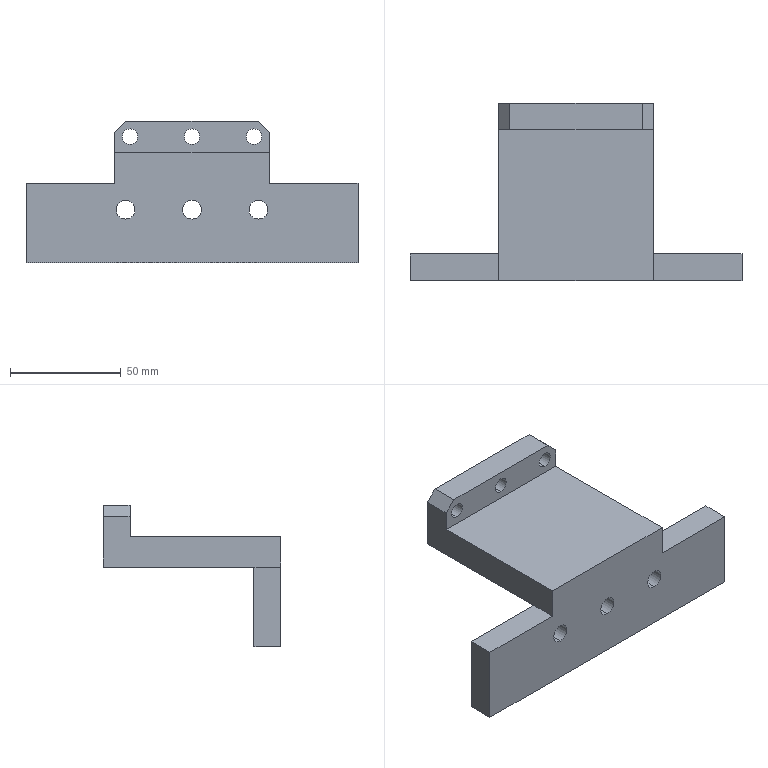NC program | NX | posted with a generic post | part box 150 x 80 x 64 mm
Lines 1 to 22 of 10576:
N10 G17 G21 G94 G90
(FLOOR_WALL , TOOL : D63)
N12 T01 M6
N14 G54
N16 G17 G0 G90 X-113. Y43.497 B0. C0. S6500 M3
N18 G43 Z30. H1
N20 Z3.
N22 G94 G1 Z0. F1250.
N24 X-110.
N26 X110.
N28 Y12.599
N30 X-110.
N32 Y-18.3
N34 X110.
N36 X113.
N38 Z3.
N40 G0 Z30.
N42 M5